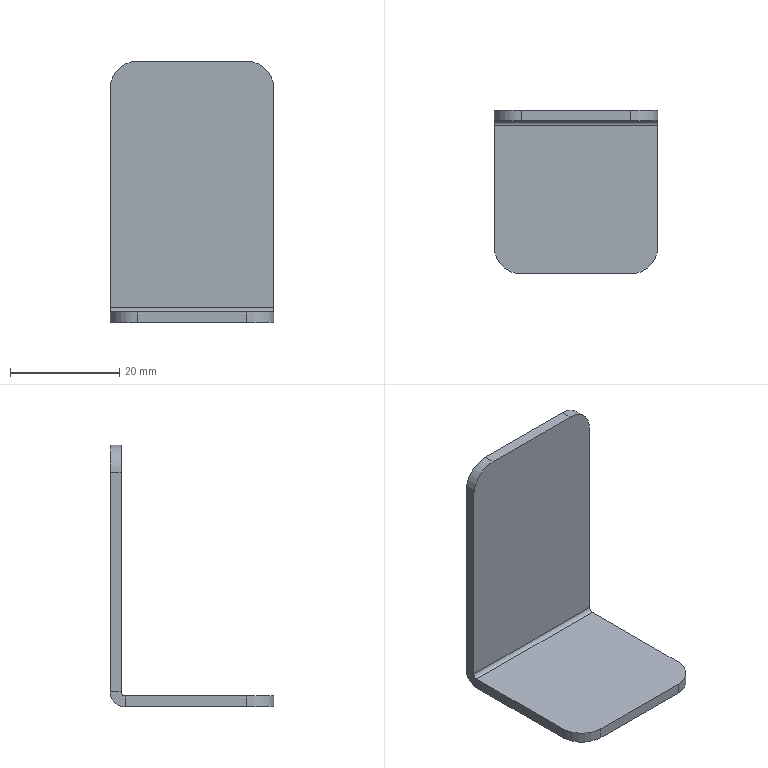Part | SolidWorks | features EdgeFlange 1, Fillet 1, FlatPattern 1, SMBaseFlange 1, SheetMetal 1 | 1 solid | 18 faces | box 30 x 30 x 48 mm | volume 4472 mm3 | plane 12 | cylinder 6 | commonest cylinder face diameters 10 x4 1.473 x1 5.473 x1
STEP:
#1=CARTESIAN_POINT('',(-15.,12.263,-2.));
#2=VERTEX_POINT('',#1);
#3=CARTESIAN_POINT('',(-15.,-10.,-2.));
#4=VERTEX_POINT('',#3);
#5=CARTESIAN_POINT('',(-15.,15.,-2.));
#6=DIRECTION('',(0.,-1.,0.));
#7=VECTOR('',#6,1000.);
#8=LINE('',#5,#7);
#9=EDGE_CURVE('',#2,#4,#8,.T.);
#10=ORIENTED_EDGE('',*,*,#9,.T.);
#11=CARTESIAN_POINT('',(-15.,-10.,0.));
#12=VERTEX_POINT('',#11);
#13=CARTESIAN_POINT('',(-15.,-10.,-2.));
#14=DIRECTION('',(0.,0.,1.));
#15=VECTOR('',#14,1000.);
#16=LINE('',#13,#15);
#17=EDGE_CURVE('',#4,#12,#16,.T.);
#18=ORIENTED_EDGE('',*,*,#17,.T.);
#19=CARTESIAN_POINT('',(-15.,12.263,0.));
#20=VERTEX_POINT('',#19);
#21=CARTESIAN_POINT('',(-15.,15.,0.));
#22=DIRECTION('',(0.,-1.,0.));
#23=VECTOR('',#22,1000.);
#24=LINE('',#21,#23);
#25=EDGE_CURVE('',#20,#12,#24,.T.);
#26=ORIENTED_EDGE('',*,*,#25,.F.);
#27=CARTESIAN_POINT('',(-15.,12.263,0.));
#28=DIRECTION('',(0.,0.,-1.));
#29=VECTOR('',#28,1000.);
#30=LINE('',#27,#29);
#31=EDGE_CURVE('',#20,#2,#30,.T.);
#32=ORIENTED_EDGE('',*,*,#31,.T.);
#33=EDGE_LOOP('',(#10,#18,#26,#32));
#34=FACE_OUTER_BOUND('',#33,.T.);
#35=CARTESIAN_POINT('',(-15.,15.,-2.));
#36=DIRECTION('',(-1.,0.,0.));
#37=DIRECTION('',(0.,-1.,0.));
#38=AXIS2_PLACEMENT_3D('',#35,#36,#37);
#39=PLANE('',#38);
#40=ADVANCED_FACE('',(#34),#39,.T.);
#41=CARTESIAN_POINT('',(-10.,-15.,-2.));
#42=VERTEX_POINT('',#41);
#43=CARTESIAN_POINT('',(10.,-15.,-2.));
#44=VERTEX_POINT('',#43);
#45=CARTESIAN_POINT('',(-15.,-15.,-2.));
#46=DIRECTION('',(1.,0.,0.));
#47=VECTOR('',#46,1000.);
#48=LINE('',#45,#47);
#49=EDGE_CURVE('',#42,#44,#48,.T.);
#50=ORIENTED_EDGE('',*,*,#49,.F.);
#51=CARTESIAN_POINT('',(-10.,-10.,-2.));
#52=DIRECTION('',(0.,0.,-1.));
#53=DIRECTION('',(1.,0.,0.));
#54=AXIS2_PLACEMENT_3D('',#51,#52,#53);
#55=CIRCLE('',#54,5.);
#56=EDGE_CURVE('',#42,#4,#55,.T.);
#57=ORIENTED_EDGE('',*,*,#56,.T.);
#58=ORIENTED_EDGE('',*,*,#9,.F.);
#59=CARTESIAN_POINT('',(15.,12.263,-2.));
#60=VERTEX_POINT('',#59);
#61=CARTESIAN_POINT('',(-15.,12.263,-2.));
#62=DIRECTION('',(1.,0.,0.));
#63=VECTOR('',#62,1000.);
#64=LINE('',#61,#63);
#65=EDGE_CURVE('',#2,#60,#64,.T.);
#66=ORIENTED_EDGE('',*,*,#65,.T.);
#67=CARTESIAN_POINT('',(15.,-10.,-2.));
#68=VERTEX_POINT('',#67);
#69=CARTESIAN_POINT('',(15.,15.,-2.));
#70=DIRECTION('',(0.,1.,0.));
#71=VECTOR('',#70,1000.);
#72=LINE('',#69,#71);
#73=EDGE_CURVE('',#68,#60,#72,.T.);
#74=ORIENTED_EDGE('',*,*,#73,.F.);
#75=CARTESIAN_POINT('',(10.,-10.,-2.));
#76=DIRECTION('',(0.,0.,-1.));
#77=DIRECTION('',(1.,0.,0.));
#78=AXIS2_PLACEMENT_3D('',#75,#76,#77);
#79=CIRCLE('',#78,5.);
#80=EDGE_CURVE('',#68,#44,#79,.T.);
#81=ORIENTED_EDGE('',*,*,#80,.T.);
#82=EDGE_LOOP('',(#50,#57,#58,#66,#74,#81));
#83=FACE_OUTER_BOUND('',#82,.T.);
#84=CARTESIAN_POINT('',(0.,0.,-2.));
#85=DIRECTION('',(0.,0.,1.));
#86=DIRECTION('',(1.,0.,0.));
#87=AXIS2_PLACEMENT_3D('',#84,#85,#86);
#88=PLANE('',#87);
#89=ADVANCED_FACE('',(#83),#88,.F.);
#90=ORIENTED_EDGE('',*,*,#25,.T.);
#91=CARTESIAN_POINT('',(-10.,-15.,0.));
#92=VERTEX_POINT('',#91);
#93=CARTESIAN_POINT('',(-10.,-10.,0.));
#94=DIRECTION('',(0.,0.,1.));
#95=DIRECTION('',(1.,0.,0.));
#96=AXIS2_PLACEMENT_3D('',#93,#94,#95);
#97=CIRCLE('',#96,5.);
#98=EDGE_CURVE('',#12,#92,#97,.T.);
#99=ORIENTED_EDGE('',*,*,#98,.T.);
#100=CARTESIAN_POINT('',(10.,-15.,0.));
#101=VERTEX_POINT('',#100);
#102=CARTESIAN_POINT('',(-15.,-15.,0.));
#103=DIRECTION('',(1.,0.,0.));
#104=VECTOR('',#103,1000.);
#105=LINE('',#102,#104);
#106=EDGE_CURVE('',#92,#101,#105,.T.);
#107=ORIENTED_EDGE('',*,*,#106,.T.);
#108=CARTESIAN_POINT('',(15.,-10.,0.));
#109=VERTEX_POINT('',#108);
#110=CARTESIAN_POINT('',(10.,-10.,0.));
#111=DIRECTION('',(0.,0.,1.));
#112=DIRECTION('',(1.,0.,0.));
#113=AXIS2_PLACEMENT_3D('',#110,#111,#112);
#114=CIRCLE('',#113,5.);
#115=EDGE_CURVE('',#101,#109,#114,.T.);
#116=ORIENTED_EDGE('',*,*,#115,.T.);
#117=CARTESIAN_POINT('',(15.,12.263,0.));
#118=VERTEX_POINT('',#117);
#119=CARTESIAN_POINT('',(15.,15.,0.));
#120=DIRECTION('',(0.,1.,0.));
#121=VECTOR('',#120,1000.);
#122=LINE('',#119,#121);
#123=EDGE_CURVE('',#109,#118,#122,.T.);
#124=ORIENTED_EDGE('',*,*,#123,.T.);
#125=CARTESIAN_POINT('',(-15.,12.263,0.));
#126=DIRECTION('',(1.,0.,0.));
#127=VECTOR('',#126,1000.);
#128=LINE('',#125,#127);
#129=EDGE_CURVE('',#20,#118,#128,.T.);
#130=ORIENTED_EDGE('',*,*,#129,.F.);
#131=EDGE_LOOP('',(#90,#99,#107,#116,#124,#130));
#132=FACE_OUTER_BOUND('',#131,.T.);
#133=CARTESIAN_POINT('',(0.,0.,0.));
#134=DIRECTION('',(0.,0.,1.));
#135=DIRECTION('',(1.,0.,0.));
#136=AXIS2_PLACEMENT_3D('',#133,#134,#135);
#137=PLANE('',#136);
#138=ADVANCED_FACE('',(#132),#137,.T.);
#139=ORIENTED_EDGE('',*,*,#123,.F.);
#140=CARTESIAN_POINT('',(15.,-10.,-2.));
#141=DIRECTION('',(0.,0.,-1.));
#142=VECTOR('',#141,1000.);
#143=LINE('',#140,#142);
#144=EDGE_CURVE('',#109,#68,#143,.T.);
#145=ORIENTED_EDGE('',*,*,#144,.T.);
#146=ORIENTED_EDGE('',*,*,#73,.T.);
#147=CARTESIAN_POINT('',(15.,12.263,0.));
#148=DIRECTION('',(0.,0.,-1.));
#149=VECTOR('',#148,1000.);
#150=LINE('',#147,#149);
#151=EDGE_CURVE('',#118,#60,#150,.T.);
#152=ORIENTED_EDGE('',*,*,#151,.F.);
#153=EDGE_LOOP('',(#139,#145,#146,#152));
#154=FACE_OUTER_BOUND('',#153,.T.);
#155=CARTESIAN_POINT('',(15.,15.,-2.));
#156=DIRECTION('',(1.,0.,0.));
#157=DIRECTION('',(0.,1.,0.));
#158=AXIS2_PLACEMENT_3D('',#155,#156,#157);
#159=PLANE('',#158);
#160=ADVANCED_FACE('',(#154),#159,.T.);
#161=ORIENTED_EDGE('',*,*,#106,.F.);
#162=CARTESIAN_POINT('',(-10.,-15.,-2.));
#163=DIRECTION('',(0.,0.,-1.));
#164=VECTOR('',#163,1000.);
#165=LINE('',#162,#164);
#166=EDGE_CURVE('',#92,#42,#165,.T.);
#167=ORIENTED_EDGE('',*,*,#166,.T.);
#168=ORIENTED_EDGE('',*,*,#49,.T.);
#169=CARTESIAN_POINT('',(10.,-15.,-2.));
#170=DIRECTION('',(0.,0.,1.));
#171=VECTOR('',#170,1000.);
#172=LINE('',#169,#171);
#173=EDGE_CURVE('',#44,#101,#172,.T.);
#174=ORIENTED_EDGE('',*,*,#173,.T.);
#175=EDGE_LOOP('',(#161,#167,#168,#174));
#176=FACE_OUTER_BOUND('',#175,.T.);
#177=CARTESIAN_POINT('',(-15.,-15.,-2.));
#178=DIRECTION('',(0.,-1.,0.));
#179=DIRECTION('',(0.,0.,-1.));
#180=AXIS2_PLACEMENT_3D('',#177,#178,#179);
#181=PLANE('',#180);
#182=ADVANCED_FACE('',(#176),#181,.T.);
#183=CARTESIAN_POINT('',(15.,13.,0.7366));
#184=VERTEX_POINT('',#183);
#185=CARTESIAN_POINT('',(15.,15.,0.7366));
#186=VERTEX_POINT('',#185);
#187=CARTESIAN_POINT('',(15.,15.,0.7366));
#188=DIRECTION('',(0.,1.,0.));
#189=VECTOR('',#188,1000.);
#190=LINE('',#187,#189);
#191=EDGE_CURVE('',#184,#186,#190,.T.);
#192=ORIENTED_EDGE('',*,*,#191,.F.);
#193=CARTESIAN_POINT('',(15.,12.263,0.7366));
#194=DIRECTION('',(1.,0.,0.));
#195=DIRECTION('',(0.,0.,1.));
#196=AXIS2_PLACEMENT_3D('',#193,#194,#195);
#197=CIRCLE('',#196,0.7366);
#198=EDGE_CURVE('',#118,#184,#197,.T.);
#199=ORIENTED_EDGE('',*,*,#198,.F.);
#200=ORIENTED_EDGE('',*,*,#151,.T.);
#201=CARTESIAN_POINT('',(15.,12.263,0.7366));
#202=DIRECTION('',(1.,0.,0.));
#203=DIRECTION('',(0.,0.,1.));
#204=AXIS2_PLACEMENT_3D('',#201,#202,#203);
#205=CIRCLE('',#204,2.737);
#206=EDGE_CURVE('',#60,#186,#205,.T.);
#207=ORIENTED_EDGE('',*,*,#206,.T.);
#208=EDGE_LOOP('',(#192,#199,#200,#207));
#209=FACE_OUTER_BOUND('',#208,.T.);
#210=CARTESIAN_POINT('',(15.,12.263,0.7366));
#211=DIRECTION('',(1.,0.,0.));
#212=DIRECTION('',(0.,0.,-1.));
#213=AXIS2_PLACEMENT_3D('',#210,#211,#212);
#214=PLANE('',#213);
#215=ADVANCED_FACE('',(#209),#214,.T.);
#216=CARTESIAN_POINT('',(-15.,13.,0.7366));
#217=VERTEX_POINT('',#216);
#218=CARTESIAN_POINT('',(-15.,12.263,0.7366));
#219=DIRECTION('',(-1.,0.,0.));
#220=DIRECTION('',(0.,0.,1.));
#221=AXIS2_PLACEMENT_3D('',#218,#219,#220);
#222=CIRCLE('',#221,0.7366);
#223=EDGE_CURVE('',#217,#20,#222,.T.);
#224=ORIENTED_EDGE('',*,*,#223,.F.);
#225=CARTESIAN_POINT('',(-15.,15.,0.7366));
#226=VERTEX_POINT('',#225);
#227=CARTESIAN_POINT('',(-15.,13.,0.7366));
#228=DIRECTION('',(0.,1.,0.));
#229=VECTOR('',#228,1000.);
#230=LINE('',#227,#229);
#231=EDGE_CURVE('',#217,#226,#230,.T.);
#232=ORIENTED_EDGE('',*,*,#231,.T.);
#233=CARTESIAN_POINT('',(-15.,12.263,0.7366));
#234=DIRECTION('',(-1.,0.,0.));
#235=DIRECTION('',(0.,0.,1.));
#236=AXIS2_PLACEMENT_3D('',#233,#234,#235);
#237=CIRCLE('',#236,2.737);
#238=EDGE_CURVE('',#226,#2,#237,.T.);
#239=ORIENTED_EDGE('',*,*,#238,.T.);
#240=ORIENTED_EDGE('',*,*,#31,.F.);
#241=EDGE_LOOP('',(#224,#232,#239,#240));
#242=FACE_OUTER_BOUND('',#241,.T.);
#243=CARTESIAN_POINT('',(-15.,12.263,0.7366));
#244=DIRECTION('',(1.,0.,0.));
#245=DIRECTION('',(0.,0.,-1.));
#246=AXIS2_PLACEMENT_3D('',#243,#244,#245);
#247=PLANE('',#246);
#248=ADVANCED_FACE('',(#242),#247,.F.);
#249=ORIENTED_EDGE('',*,*,#65,.F.);
#250=ORIENTED_EDGE('',*,*,#238,.F.);
#251=CARTESIAN_POINT('',(15.,15.,0.7366));
#252=DIRECTION('',(1.,0.,0.));
#253=VECTOR('',#252,1000.);
#254=LINE('',#251,#253);
#255=EDGE_CURVE('',#226,#186,#254,.T.);
#256=ORIENTED_EDGE('',*,*,#255,.T.);
#257=ORIENTED_EDGE('',*,*,#206,.F.);
#258=EDGE_LOOP('',(#249,#250,#256,#257));
#259=FACE_OUTER_BOUND('',#258,.T.);
#260=CARTESIAN_POINT('',(-15.,12.263,0.7366));
#261=DIRECTION('',(-1.,0.,0.));
#262=DIRECTION('',(0.,1.,0.));
#263=AXIS2_PLACEMENT_3D('',#260,#261,#262);
#264=CYLINDRICAL_SURFACE('',#263,2.737);
#265=ADVANCED_FACE('',(#259),#264,.T.);
#266=ORIENTED_EDGE('',*,*,#129,.T.);
#267=ORIENTED_EDGE('',*,*,#198,.T.);
#268=CARTESIAN_POINT('',(15.,13.,0.7366));
#269=DIRECTION('',(-1.,0.,0.));
#270=VECTOR('',#269,1000.);
#271=LINE('',#268,#270);
#272=EDGE_CURVE('',#184,#217,#271,.T.);
#273=ORIENTED_EDGE('',*,*,#272,.T.);
#274=ORIENTED_EDGE('',*,*,#223,.T.);
#275=EDGE_LOOP('',(#266,#267,#273,#274));
#276=FACE_OUTER_BOUND('',#275,.T.);
#277=CARTESIAN_POINT('',(-15.,12.263,0.7366));
#278=DIRECTION('',(-1.,0.,0.));
#279=DIRECTION('',(0.,1.,0.));
#280=AXIS2_PLACEMENT_3D('',#277,#278,#279);
#281=CYLINDRICAL_SURFACE('',#280,0.7366);
#282=ADVANCED_FACE('',(#276),#281,.F.);
#283=CARTESIAN_POINT('',(15.,15.,41.));
#284=VERTEX_POINT('',#283);
#285=CARTESIAN_POINT('',(15.,15.,0.));
#286=DIRECTION('',(0.,0.,-1.));
#287=VECTOR('',#286,1000.);
#288=LINE('',#285,#287);
#289=EDGE_CURVE('',#284,#186,#288,.T.);
#290=ORIENTED_EDGE('',*,*,#289,.F.);
#291=CARTESIAN_POINT('',(15.,13.,41.));
#292=VERTEX_POINT('',#291);
#293=CARTESIAN_POINT('',(15.,15.,41.));
#294=DIRECTION('',(0.,-1.,0.));
#295=VECTOR('',#294,1000.);
#296=LINE('',#293,#295);
#297=EDGE_CURVE('',#284,#292,#296,.T.);
#298=ORIENTED_EDGE('',*,*,#297,.T.);
#299=CARTESIAN_POINT('',(15.,13.,0.));
#300=DIRECTION('',(0.,0.,-1.));
#301=VECTOR('',#300,1000.);
#302=LINE('',#299,#301);
#303=EDGE_CURVE('',#292,#184,#302,.T.);
#304=ORIENTED_EDGE('',*,*,#303,.T.);
#305=ORIENTED_EDGE('',*,*,#191,.T.);
#306=EDGE_LOOP('',(#290,#298,#304,#305));
#307=FACE_OUTER_BOUND('',#306,.T.);
#308=CARTESIAN_POINT('',(15.,15.,0.));
#309=DIRECTION('',(-1.,0.,0.));
#310=DIRECTION('',(0.,0.,1.));
#311=AXIS2_PLACEMENT_3D('',#308,#309,#310);
#312=PLANE('',#311);
#313=ADVANCED_FACE('',(#307),#312,.F.);
#314=CARTESIAN_POINT('',(-15.,13.,41.));
#315=VERTEX_POINT('',#314);
#316=CARTESIAN_POINT('',(-15.,13.,46.));
#317=DIRECTION('',(0.,0.,1.));
#318=VECTOR('',#317,1000.);
#319=LINE('',#316,#318);
#320=EDGE_CURVE('',#217,#315,#319,.T.);
#321=ORIENTED_EDGE('',*,*,#320,.T.);
#322=CARTESIAN_POINT('',(-15.,15.,41.));
#323=VERTEX_POINT('',#322);
#324=CARTESIAN_POINT('',(-15.,15.,41.));
#325=DIRECTION('',(0.,1.,0.));
#326=VECTOR('',#325,1000.);
#327=LINE('',#324,#326);
#328=EDGE_CURVE('',#315,#323,#327,.T.);
#329=ORIENTED_EDGE('',*,*,#328,.T.);
#330=CARTESIAN_POINT('',(-15.,15.,0.));
#331=DIRECTION('',(0.,0.,1.));
#332=VECTOR('',#331,1000.);
#333=LINE('',#330,#332);
#334=EDGE_CURVE('',#226,#323,#333,.T.);
#335=ORIENTED_EDGE('',*,*,#334,.F.);
#336=ORIENTED_EDGE('',*,*,#231,.F.);
#337=EDGE_LOOP('',(#321,#329,#335,#336));
#338=FACE_OUTER_BOUND('',#337,.T.);
#339=CARTESIAN_POINT('',(-15.,15.,46.));
#340=DIRECTION('',(1.,0.,0.));
#341=DIRECTION('',(0.,0.,-1.));
#342=AXIS2_PLACEMENT_3D('',#339,#340,#341);
#343=PLANE('',#342);
#344=ADVANCED_FACE('',(#338),#343,.F.);
#345=CARTESIAN_POINT('',(-10.,15.,46.));
#346=VERTEX_POINT('',#345);
#347=CARTESIAN_POINT('',(10.,15.,46.));
#348=VERTEX_POINT('',#347);
#349=CARTESIAN_POINT('',(0.,15.,46.));
#350=DIRECTION('',(1.,0.,0.));
#351=VECTOR('',#350,1000.);
#352=LINE('',#349,#351);
#353=EDGE_CURVE('',#346,#348,#352,.T.);
#354=ORIENTED_EDGE('',*,*,#353,.T.);
#355=CARTESIAN_POINT('',(10.,15.,41.));
#356=DIRECTION('',(0.,1.,0.));
#357=DIRECTION('',(0.,0.,-1.));
#358=AXIS2_PLACEMENT_3D('',#355,#356,#357);
#359=CIRCLE('',#358,5.);
#360=EDGE_CURVE('',#348,#284,#359,.T.);
#361=ORIENTED_EDGE('',*,*,#360,.T.);
#362=ORIENTED_EDGE('',*,*,#289,.T.);
#363=ORIENTED_EDGE('',*,*,#255,.F.);
#364=ORIENTED_EDGE('',*,*,#334,.T.);
#365=CARTESIAN_POINT('',(-10.,15.,41.));
#366=DIRECTION('',(0.,1.,0.));
#367=DIRECTION('',(0.,0.,-1.));
#368=AXIS2_PLACEMENT_3D('',#365,#366,#367);
#369=CIRCLE('',#368,5.);
#370=EDGE_CURVE('',#323,#346,#369,.T.);
#371=ORIENTED_EDGE('',*,*,#370,.T.);
#372=EDGE_LOOP('',(#354,#361,#362,#363,#364,#371));
#373=FACE_OUTER_BOUND('',#372,.T.);
#374=CARTESIAN_POINT('',(0.,15.,0.));
#375=DIRECTION('',(0.,-1.,0.));
#376=DIRECTION('',(0.,0.,-1.));
#377=AXIS2_PLACEMENT_3D('',#374,#375,#376);
#378=PLANE('',#377);
#379=ADVANCED_FACE('',(#373),#378,.F.);
#380=ORIENTED_EDGE('',*,*,#303,.F.);
#381=CARTESIAN_POINT('',(10.,13.,46.));
#382=VERTEX_POINT('',#381);
#383=CARTESIAN_POINT('',(10.,13.,41.));
#384=DIRECTION('',(0.,-1.,0.));
#385=DIRECTION('',(0.,0.,-1.));
#386=AXIS2_PLACEMENT_3D('',#383,#384,#385);
#387=CIRCLE('',#386,5.);
#388=EDGE_CURVE('',#292,#382,#387,.T.);
#389=ORIENTED_EDGE('',*,*,#388,.T.);
#390=CARTESIAN_POINT('',(-10.,13.,46.));
#391=VERTEX_POINT('',#390);
#392=CARTESIAN_POINT('',(15.,13.,46.));
#393=DIRECTION('',(1.,0.,0.));
#394=VECTOR('',#393,1000.);
#395=LINE('',#392,#394);
#396=EDGE_CURVE('',#391,#382,#395,.T.);
#397=ORIENTED_EDGE('',*,*,#396,.F.);
#398=CARTESIAN_POINT('',(-10.,13.,41.));
#399=DIRECTION('',(0.,-1.,0.));
#400=DIRECTION('',(0.,0.,-1.));
#401=AXIS2_PLACEMENT_3D('',#398,#399,#400);
#402=CIRCLE('',#401,5.);
#403=EDGE_CURVE('',#391,#315,#402,.T.);
#404=ORIENTED_EDGE('',*,*,#403,.T.);
#405=ORIENTED_EDGE('',*,*,#320,.F.);
#406=ORIENTED_EDGE('',*,*,#272,.F.);
#407=EDGE_LOOP('',(#380,#389,#397,#404,#405,#406));
#408=FACE_OUTER_BOUND('',#407,.T.);
#409=CARTESIAN_POINT('',(0.,13.,0.));
#410=DIRECTION('',(0.,-1.,0.));
#411=DIRECTION('',(0.,0.,-1.));
#412=AXIS2_PLACEMENT_3D('',#409,#410,#411);
#413=PLANE('',#412);
#414=ADVANCED_FACE('',(#408),#413,.T.);
#415=ORIENTED_EDGE('',*,*,#396,.T.);
#416=CARTESIAN_POINT('',(10.,15.,46.));
#417=DIRECTION('',(0.,1.,0.));
#418=VECTOR('',#417,1000.);
#419=LINE('',#416,#418);
#420=EDGE_CURVE('',#382,#348,#419,.T.);
#421=ORIENTED_EDGE('',*,*,#420,.T.);
#422=ORIENTED_EDGE('',*,*,#353,.F.);
#423=CARTESIAN_POINT('',(-10.,15.,46.));
#424=DIRECTION('',(0.,-1.,0.));
#425=VECTOR('',#424,1000.);
#426=LINE('',#423,#425);
#427=EDGE_CURVE('',#346,#391,#426,.T.);
#428=ORIENTED_EDGE('',*,*,#427,.T.);
#429=EDGE_LOOP('',(#415,#421,#422,#428));
#430=FACE_OUTER_BOUND('',#429,.T.);
#431=CARTESIAN_POINT('',(15.,15.,46.));
#432=DIRECTION('',(0.,0.,-1.));
#433=DIRECTION('',(0.,1.,0.));
#434=AXIS2_PLACEMENT_3D('',#431,#432,#433);
#435=PLANE('',#434);
#436=ADVANCED_FACE('',(#430),#435,.F.);
#437=ORIENTED_EDGE('',*,*,#56,.F.);
#438=ORIENTED_EDGE('',*,*,#166,.F.);
#439=ORIENTED_EDGE('',*,*,#98,.F.);
#440=ORIENTED_EDGE('',*,*,#17,.F.);
#441=EDGE_LOOP('',(#437,#438,#439,#440));
#442=FACE_OUTER_BOUND('',#441,.T.);
#443=CARTESIAN_POINT('',(-10.,-10.,-2.));
#444=DIRECTION('',(0.,0.,1.));
#445=DIRECTION('',(1.,0.,0.));
#446=AXIS2_PLACEMENT_3D('',#443,#444,#445);
#447=CYLINDRICAL_SURFACE('',#446,5.);
#448=ADVANCED_FACE('',(#442),#447,.T.);
#449=ORIENTED_EDGE('',*,*,#80,.F.);
#450=ORIENTED_EDGE('',*,*,#144,.F.);
#451=ORIENTED_EDGE('',*,*,#115,.F.);
#452=ORIENTED_EDGE('',*,*,#173,.F.);
#453=EDGE_LOOP('',(#449,#450,#451,#452));
#454=FACE_OUTER_BOUND('',#453,.T.);
#455=CARTESIAN_POINT('',(10.,-10.,-2.));
#456=DIRECTION('',(0.,0.,1.));
#457=DIRECTION('',(1.,0.,0.));
#458=AXIS2_PLACEMENT_3D('',#455,#456,#457);
#459=CYLINDRICAL_SURFACE('',#458,5.);
#460=ADVANCED_FACE('',(#454),#459,.T.);
#461=ORIENTED_EDGE('',*,*,#360,.F.);
#462=ORIENTED_EDGE('',*,*,#420,.F.);
#463=ORIENTED_EDGE('',*,*,#388,.F.);
#464=ORIENTED_EDGE('',*,*,#297,.F.);
#465=EDGE_LOOP('',(#461,#462,#463,#464));
#466=FACE_OUTER_BOUND('',#465,.T.);
#467=CARTESIAN_POINT('',(10.,15.,41.));
#468=DIRECTION('',(0.,-1.,0.));
#469=DIRECTION('',(0.,0.,-1.));
#470=AXIS2_PLACEMENT_3D('',#467,#468,#469);
#471=CYLINDRICAL_SURFACE('',#470,5.);
#472=ADVANCED_FACE('',(#466),#471,.T.);
#473=ORIENTED_EDGE('',*,*,#370,.F.);
#474=ORIENTED_EDGE('',*,*,#328,.F.);
#475=ORIENTED_EDGE('',*,*,#403,.F.);
#476=ORIENTED_EDGE('',*,*,#427,.F.);
#477=EDGE_LOOP('',(#473,#474,#475,#476));
#478=FACE_OUTER_BOUND('',#477,.T.);
#479=CARTESIAN_POINT('',(-10.,15.,41.));
#480=DIRECTION('',(0.,-1.,0.));
#481=DIRECTION('',(0.,0.,-1.));
#482=AXIS2_PLACEMENT_3D('',#479,#480,#481);
#483=CYLINDRICAL_SURFACE('',#482,5.);
#484=ADVANCED_FACE('',(#478),#483,.T.);
#485=CLOSED_SHELL('',(#40,#89,#138,#160,#182,#215,#248,#265,#282,#313,#344,#379,#414,#436,#448,#460,#472,#484));
#486=MANIFOLD_SOLID_BREP('',#485);
#487=CARTESIAN_POINT('',(0.,0.,0.));
#488=DIRECTION('',(0.,0.,1.));
#489=DIRECTION('',(1.,0.,0.));
#490=AXIS2_PLACEMENT_3D('',#487,#488,#489);
#491=(LENGTH_UNIT()NAMED_UNIT(*)SI_UNIT(.MILLI.,.METRE.));
#492=UNCERTAINTY_MEASURE_WITH_UNIT(LENGTH_MEASURE(0.00001),#491,'','');
#493=(NAMED_UNIT(*)PLANE_ANGLE_UNIT()SI_UNIT($,.RADIAN.));
#494=(NAMED_UNIT(*)SI_UNIT($,.STERADIAN.)SOLID_ANGLE_UNIT());
#495=(GEOMETRIC_REPRESENTATION_CONTEXT(3)GLOBAL_UNCERTAINTY_ASSIGNED_CONTEXT((#492))GLOBAL_UNIT_ASSIGNED_CONTEXT((#491,#493,#494))REPRESENTATION_CONTEXT('',''));
#496=ADVANCED_BREP_SHAPE_REPRESENTATION('',(#486,#490),#495);